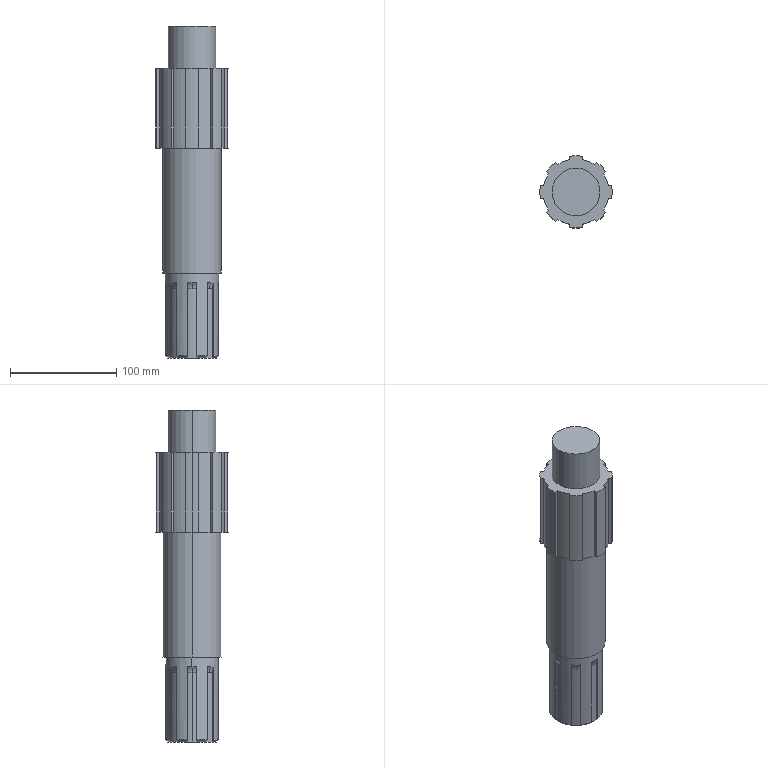Part | SolidWorks | features ICE 4, Chamfer 1, CirPattern 1, Extrusion 1, SweepCut 1 | 1 solid | 93 faces | box 68 x 68 x 312.5 mm | volume 737851 mm3 | plane 37 | cylinder 32 | torus 16 | cone 8 | commonest cylinder face diameters 46 x9 68 x9 62 x8 45 x2 50 x2 55 x2